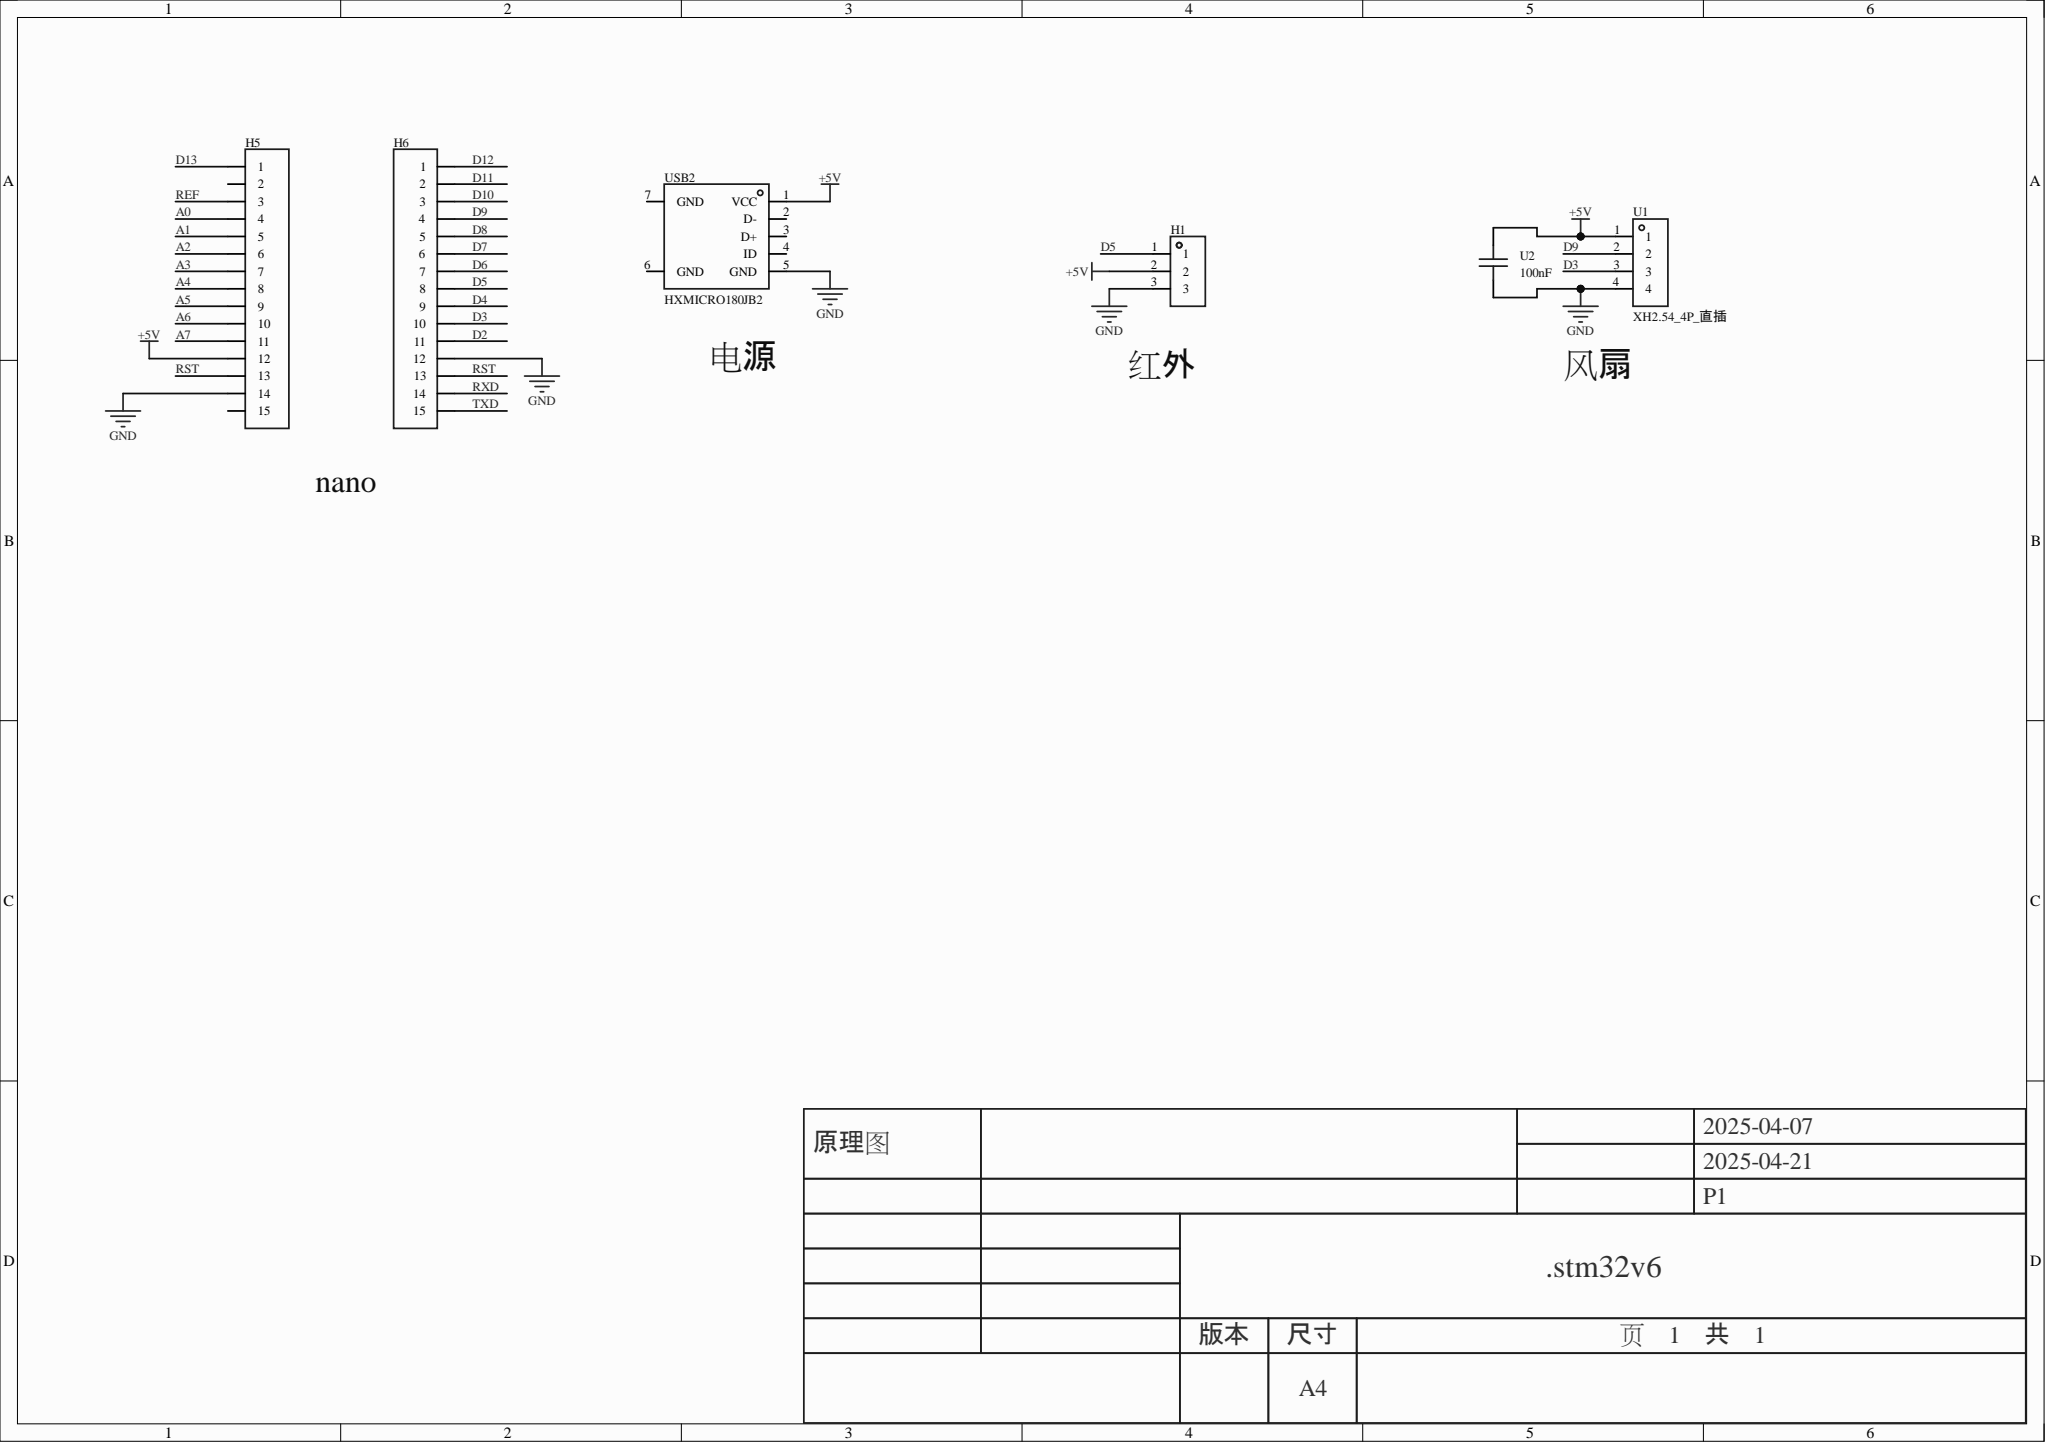Circuit board | Altium Designer | 6 parts | 6 nets
Bill of materials:
Comment,Description,Designator,Footprint,LibRef,Quantity
"","","H1","HDR-TH_3P-P2.54-V-F","HDR-F_2.54_1x3P","1"
"","","H5, H6","HDR-TH_15P-P2.54-V-F-1","HDR-F_2.54_1x15P","2"
"XH2.54_4P_直插","","U1","CONN-TH_4P-P2.50-XH2.54-4P","XH2.54_4P_直插","1"
"100nF","","U2","CAP-TH_L5.0-W2.5-P5.00-D1.0","100nF","1"
"HXMICRO180JB2","","USB2","MICRO-USB-TH_HXMICRO180JB2","HXMICRO180JB2","1"
Netlist (Protel format):
[
H1
HDR-TH_3P-P2.54-V-F




]
[
H5
HDR-TH_15P-P2.54-V-F-1




]
[
H6
HDR-TH_15P-P2.54-V-F-1




]
[
U1
CONN-TH_4P-P2.50-XH2.54-4P
XH2.54_4P_直插



]
[
U2
CAP-TH_L5.0-W2.5-P5.00-D1.0
100nF



]
[
USB2
MICRO-USB-TH_HXMICRO180JB2
HXMICRO180JB2



]
(
RST
H5-13
H6-13
)
(
GND
H1-3
H5-14
H6-12
U1-4
U2-2
USB2-5
)
(
D9
H6-4
U1-2
)
(
D5
H1-1
H6-8
)
(
D3
H6-10
U1-3
)
(
+5V
H1-2
H5-12
U1-1
U2-1
USB2-1
)